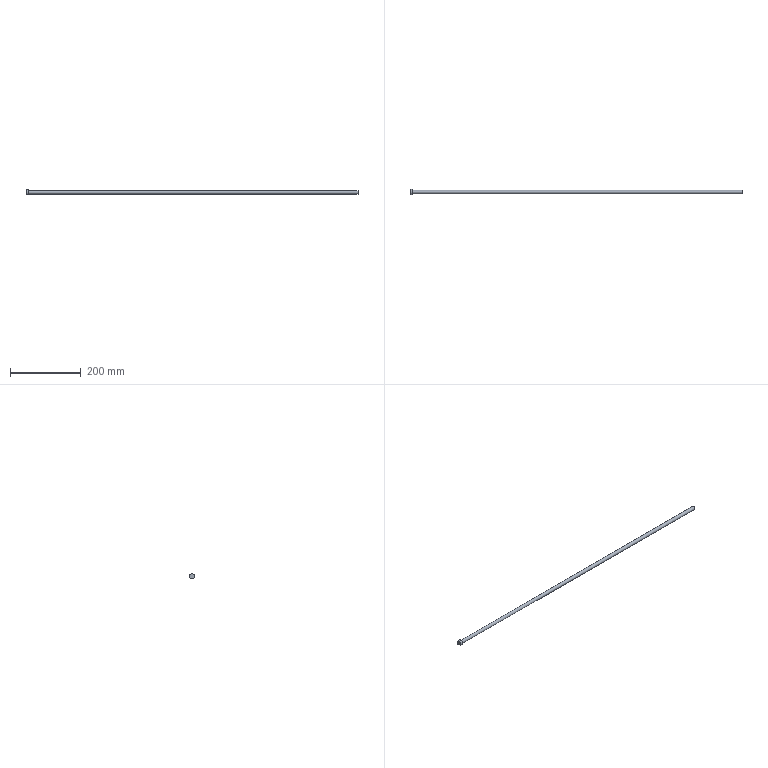Part | STEP file | solid 36 | 1 solid | 6 faces | box 940 x 15 x 13 mm | volume 74501 mm3 | plane 4 | cylinder 2 | commonest cylinder face diameters 10 x1 15 x1